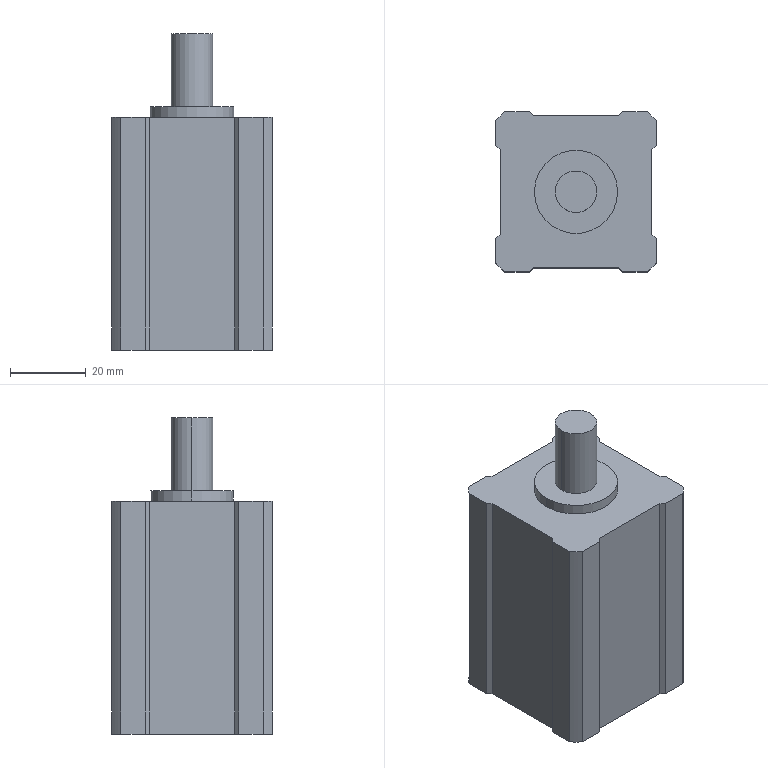Part | SolidWorks | features ICE 5, CirPattern 1, Extrusion 1, RefAxis 1, Scale 1 | 1 solid | 32 faces | box 42.35 x 42.35 x 83.6 mm | volume 106285 mm3 | plane 24 | cylinder 8 | commonest cylinder face diameters 56.65 x4 11 x2 22 x2
STEP:
#1=CARTESIAN_POINT('',(5.5,0.,109.667));
#2=VERTEX_POINT('',#1);
#3=CARTESIAN_POINT('',(-5.5,0.,109.667));
#4=VERTEX_POINT('',#3);
#5=CARTESIAN_POINT('',(0.,0.,109.667));
#6=DIRECTION('',(0.,0.,1.));
#7=DIRECTION('',(1.,0.,0.));
#8=AXIS2_PLACEMENT_3D('',#5,#6,#7);
#9=CIRCLE('',#8,5.5);
#10=EDGE_CURVE('',#2,#4,#9,.T.);
#11=ORIENTED_EDGE('',*,*,#10,.F.);
#12=CARTESIAN_POINT('',(5.5,0.,90.417));
#13=VERTEX_POINT('',#12);
#14=CARTESIAN_POINT('',(5.5,0.,109.667));
#15=DIRECTION('',(0.,0.,-1.));
#16=VECTOR('',#15,1000.);
#17=LINE('',#14,#16);
#18=EDGE_CURVE('',#2,#13,#17,.T.);
#19=ORIENTED_EDGE('',*,*,#18,.T.);
#20=CARTESIAN_POINT('',(-5.5,0.,90.417));
#21=VERTEX_POINT('',#20);
#22=CARTESIAN_POINT('',(0.,0.,90.417));
#23=DIRECTION('',(0.,0.,1.));
#24=DIRECTION('',(1.,0.,0.));
#25=AXIS2_PLACEMENT_3D('',#22,#23,#24);
#26=CIRCLE('',#25,5.5);
#27=EDGE_CURVE('',#13,#21,#26,.T.);
#28=ORIENTED_EDGE('',*,*,#27,.T.);
#29=CARTESIAN_POINT('',(-5.5,0.,109.667));
#30=DIRECTION('',(0.,0.,-1.));
#31=VECTOR('',#30,1000.);
#32=LINE('',#29,#31);
#33=EDGE_CURVE('',#4,#21,#32,.T.);
#34=ORIENTED_EDGE('',*,*,#33,.F.);
#35=EDGE_LOOP('',(#11,#19,#28,#34));
#36=FACE_OUTER_BOUND('',#35,.T.);
#37=CARTESIAN_POINT('',(0.,0.,109.667));
#38=DIRECTION('',(0.,0.,-1.));
#39=DIRECTION('',(-1.,0.,0.));
#40=AXIS2_PLACEMENT_3D('',#37,#38,#39);
#41=CYLINDRICAL_SURFACE('',#40,5.5);
#42=ADVANCED_FACE('',(#36),#41,.T.);
#43=CARTESIAN_POINT('',(11.,0.,90.417));
#44=VERTEX_POINT('',#43);
#45=CARTESIAN_POINT('',(-11.,0.,90.417));
#46=VERTEX_POINT('',#45);
#47=CARTESIAN_POINT('',(0.,0.,90.417));
#48=DIRECTION('',(0.,0.,1.));
#49=DIRECTION('',(1.,0.,0.));
#50=AXIS2_PLACEMENT_3D('',#47,#48,#49);
#51=CIRCLE('',#50,11.);
#52=EDGE_CURVE('',#44,#46,#51,.T.);
#53=ORIENTED_EDGE('',*,*,#52,.F.);
#54=CARTESIAN_POINT('',(11.,0.,87.667));
#55=VERTEX_POINT('',#54);
#56=CARTESIAN_POINT('',(11.,0.,90.417));
#57=DIRECTION('',(0.,0.,-1.));
#58=VECTOR('',#57,1000.);
#59=LINE('',#56,#58);
#60=EDGE_CURVE('',#44,#55,#59,.T.);
#61=ORIENTED_EDGE('',*,*,#60,.T.);
#62=CARTESIAN_POINT('',(-11.,0.,87.667));
#63=VERTEX_POINT('',#62);
#64=CARTESIAN_POINT('',(0.,0.,87.667));
#65=DIRECTION('',(0.,0.,1.));
#66=DIRECTION('',(1.,0.,0.));
#67=AXIS2_PLACEMENT_3D('',#64,#65,#66);
#68=CIRCLE('',#67,11.);
#69=EDGE_CURVE('',#55,#63,#68,.T.);
#70=ORIENTED_EDGE('',*,*,#69,.T.);
#71=CARTESIAN_POINT('',(-11.,0.,90.417));
#72=DIRECTION('',(0.,0.,-1.));
#73=VECTOR('',#72,1000.);
#74=LINE('',#71,#73);
#75=EDGE_CURVE('',#46,#63,#74,.T.);
#76=ORIENTED_EDGE('',*,*,#75,.F.);
#77=EDGE_LOOP('',(#53,#61,#70,#76));
#78=FACE_OUTER_BOUND('',#77,.T.);
#79=CARTESIAN_POINT('',(0.,0.,90.417));
#80=DIRECTION('',(0.,0.,-1.));
#81=DIRECTION('',(-1.,0.,0.));
#82=AXIS2_PLACEMENT_3D('',#79,#80,#81);
#83=CYLINDRICAL_SURFACE('',#82,11.);
#84=ADVANCED_FACE('',(#78),#83,.T.);
#85=CARTESIAN_POINT('',(21.175,12.375,87.667));
#86=VERTEX_POINT('',#85);
#87=CARTESIAN_POINT('',(20.075,11.275,87.667));
#88=VERTEX_POINT('',#87);
#89=CARTESIAN_POINT('',(21.175,12.375,87.667));
#90=DIRECTION('',(-0.7071,-0.7071,0.));
#91=VECTOR('',#90,1000.);
#92=LINE('',#89,#91);
#93=EDGE_CURVE('',#86,#88,#92,.T.);
#94=ORIENTED_EDGE('',*,*,#93,.F.);
#95=CARTESIAN_POINT('',(21.175,18.813,87.667));
#96=VERTEX_POINT('',#95);
#97=CARTESIAN_POINT('',(21.175,21.175,87.667));
#98=DIRECTION('',(0.,1.,0.));
#99=VECTOR('',#98,1000.);
#100=LINE('',#97,#99);
#101=EDGE_CURVE('',#86,#96,#100,.T.);
#102=ORIENTED_EDGE('',*,*,#101,.T.);
#103=CARTESIAN_POINT('',(18.813,21.175,87.667));
#104=VERTEX_POINT('',#103);
#105=CARTESIAN_POINT('',(0.,0.,87.667));
#106=DIRECTION('',(0.,0.,1.));
#107=DIRECTION('',(1.,0.,0.));
#108=AXIS2_PLACEMENT_3D('',#105,#106,#107);
#109=CIRCLE('',#108,28.325);
#110=EDGE_CURVE('',#96,#104,#109,.T.);
#111=ORIENTED_EDGE('',*,*,#110,.T.);
#112=CARTESIAN_POINT('',(12.375,21.175,87.667));
#113=VERTEX_POINT('',#112);
#114=CARTESIAN_POINT('',(-21.175,21.175,87.667));
#115=DIRECTION('',(-1.,0.,0.));
#116=VECTOR('',#115,1000.);
#117=LINE('',#114,#116);
#118=EDGE_CURVE('',#104,#113,#117,.T.);
#119=ORIENTED_EDGE('',*,*,#118,.T.);
#120=CARTESIAN_POINT('',(11.275,20.075,87.667));
#121=VERTEX_POINT('',#120);
#122=CARTESIAN_POINT('',(12.375,21.175,87.667));
#123=DIRECTION('',(0.7071,0.7071,0.));
#124=VECTOR('',#123,1000.);
#125=LINE('',#122,#124);
#126=EDGE_CURVE('',#121,#113,#125,.T.);
#127=ORIENTED_EDGE('',*,*,#126,.F.);
#128=CARTESIAN_POINT('',(-11.275,20.075,87.667));
#129=VERTEX_POINT('',#128);
#130=CARTESIAN_POINT('',(-11.275,20.075,87.667));
#131=DIRECTION('',(1.,0.,0.));
#132=VECTOR('',#131,1000.);
#133=LINE('',#130,#132);
#134=EDGE_CURVE('',#129,#121,#133,.T.);
#135=ORIENTED_EDGE('',*,*,#134,.F.);
#136=CARTESIAN_POINT('',(-12.375,21.175,87.667));
#137=VERTEX_POINT('',#136);
#138=CARTESIAN_POINT('',(-12.375,21.175,87.667));
#139=DIRECTION('',(0.7071,-0.7071,0.));
#140=VECTOR('',#139,1000.);
#141=LINE('',#138,#140);
#142=EDGE_CURVE('',#137,#129,#141,.T.);
#143=ORIENTED_EDGE('',*,*,#142,.F.);
#144=CARTESIAN_POINT('',(-18.813,21.175,87.667));
#145=VERTEX_POINT('',#144);
#146=CARTESIAN_POINT('',(-21.175,21.175,87.667));
#147=DIRECTION('',(-1.,0.,0.));
#148=VECTOR('',#147,1000.);
#149=LINE('',#146,#148);
#150=EDGE_CURVE('',#137,#145,#149,.T.);
#151=ORIENTED_EDGE('',*,*,#150,.T.);
#152=CARTESIAN_POINT('',(-21.175,18.813,87.667));
#153=VERTEX_POINT('',#152);
#154=CARTESIAN_POINT('',(0.,0.,87.667));
#155=DIRECTION('',(0.,0.,1.));
#156=DIRECTION('',(1.,0.,0.));
#157=AXIS2_PLACEMENT_3D('',#154,#155,#156);
#158=CIRCLE('',#157,28.325);
#159=EDGE_CURVE('',#145,#153,#158,.T.);
#160=ORIENTED_EDGE('',*,*,#159,.T.);
#161=CARTESIAN_POINT('',(-21.175,12.375,87.667));
#162=VERTEX_POINT('',#161);
#163=CARTESIAN_POINT('',(-21.175,21.175,87.667));
#164=DIRECTION('',(0.,-1.,0.));
#165=VECTOR('',#164,1000.);
#166=LINE('',#163,#165);
#167=EDGE_CURVE('',#153,#162,#166,.T.);
#168=ORIENTED_EDGE('',*,*,#167,.T.);
#169=CARTESIAN_POINT('',(-20.075,11.275,87.667));
#170=VERTEX_POINT('',#169);
#171=CARTESIAN_POINT('',(-21.175,12.375,87.667));
#172=DIRECTION('',(-0.7071,0.7071,0.));
#173=VECTOR('',#172,1000.);
#174=LINE('',#171,#173);
#175=EDGE_CURVE('',#170,#162,#174,.T.);
#176=ORIENTED_EDGE('',*,*,#175,.F.);
#177=CARTESIAN_POINT('',(-20.075,-11.275,87.667));
#178=VERTEX_POINT('',#177);
#179=CARTESIAN_POINT('',(-20.075,-11.275,87.667));
#180=DIRECTION('',(0.,1.,0.));
#181=VECTOR('',#180,1000.);
#182=LINE('',#179,#181);
#183=EDGE_CURVE('',#178,#170,#182,.T.);
#184=ORIENTED_EDGE('',*,*,#183,.F.);
#185=CARTESIAN_POINT('',(-21.175,-12.375,87.667));
#186=VERTEX_POINT('',#185);
#187=CARTESIAN_POINT('',(-21.175,-12.375,87.667));
#188=DIRECTION('',(0.7071,0.7071,0.));
#189=VECTOR('',#188,1000.);
#190=LINE('',#187,#189);
#191=EDGE_CURVE('',#186,#178,#190,.T.);
#192=ORIENTED_EDGE('',*,*,#191,.F.);
#193=CARTESIAN_POINT('',(-21.175,-18.813,87.667));
#194=VERTEX_POINT('',#193);
#195=CARTESIAN_POINT('',(-21.175,21.175,87.667));
#196=DIRECTION('',(0.,-1.,0.));
#197=VECTOR('',#196,1000.);
#198=LINE('',#195,#197);
#199=EDGE_CURVE('',#186,#194,#198,.T.);
#200=ORIENTED_EDGE('',*,*,#199,.T.);
#201=CARTESIAN_POINT('',(-18.813,-21.175,87.667));
#202=VERTEX_POINT('',#201);
#203=CARTESIAN_POINT('',(0.,0.,87.667));
#204=DIRECTION('',(0.,0.,1.));
#205=DIRECTION('',(1.,0.,0.));
#206=AXIS2_PLACEMENT_3D('',#203,#204,#205);
#207=CIRCLE('',#206,28.325);
#208=EDGE_CURVE('',#194,#202,#207,.T.);
#209=ORIENTED_EDGE('',*,*,#208,.T.);
#210=CARTESIAN_POINT('',(-12.375,-21.175,87.667));
#211=VERTEX_POINT('',#210);
#212=CARTESIAN_POINT('',(-21.175,-21.175,87.667));
#213=DIRECTION('',(1.,0.,0.));
#214=VECTOR('',#213,1000.);
#215=LINE('',#212,#214);
#216=EDGE_CURVE('',#202,#211,#215,.T.);
#217=ORIENTED_EDGE('',*,*,#216,.T.);
#218=CARTESIAN_POINT('',(-11.275,-20.075,87.667));
#219=VERTEX_POINT('',#218);
#220=CARTESIAN_POINT('',(-12.375,-21.175,87.667));
#221=DIRECTION('',(-0.7071,-0.7071,0.));
#222=VECTOR('',#221,1000.);
#223=LINE('',#220,#222);
#224=EDGE_CURVE('',#219,#211,#223,.T.);
#225=ORIENTED_EDGE('',*,*,#224,.F.);
#226=CARTESIAN_POINT('',(11.275,-20.075,87.667));
#227=VERTEX_POINT('',#226);
#228=CARTESIAN_POINT('',(11.275,-20.075,87.667));
#229=DIRECTION('',(-1.,0.,0.));
#230=VECTOR('',#229,1000.);
#231=LINE('',#228,#230);
#232=EDGE_CURVE('',#227,#219,#231,.T.);
#233=ORIENTED_EDGE('',*,*,#232,.F.);
#234=CARTESIAN_POINT('',(12.375,-21.175,87.667));
#235=VERTEX_POINT('',#234);
#236=CARTESIAN_POINT('',(12.375,-21.175,87.667));
#237=DIRECTION('',(-0.7071,0.7071,0.));
#238=VECTOR('',#237,1000.);
#239=LINE('',#236,#238);
#240=EDGE_CURVE('',#235,#227,#239,.T.);
#241=ORIENTED_EDGE('',*,*,#240,.F.);
#242=CARTESIAN_POINT('',(18.813,-21.175,87.667));
#243=VERTEX_POINT('',#242);
#244=CARTESIAN_POINT('',(-21.175,-21.175,87.667));
#245=DIRECTION('',(1.,0.,0.));
#246=VECTOR('',#245,1000.);
#247=LINE('',#244,#246);
#248=EDGE_CURVE('',#235,#243,#247,.T.);
#249=ORIENTED_EDGE('',*,*,#248,.T.);
#250=CARTESIAN_POINT('',(21.175,-18.813,87.667));
#251=VERTEX_POINT('',#250);
#252=CARTESIAN_POINT('',(0.,0.,87.667));
#253=DIRECTION('',(0.,0.,1.));
#254=DIRECTION('',(1.,0.,0.));
#255=AXIS2_PLACEMENT_3D('',#252,#253,#254);
#256=CIRCLE('',#255,28.325);
#257=EDGE_CURVE('',#243,#251,#256,.T.);
#258=ORIENTED_EDGE('',*,*,#257,.T.);
#259=CARTESIAN_POINT('',(21.175,-12.375,87.667));
#260=VERTEX_POINT('',#259);
#261=CARTESIAN_POINT('',(21.175,21.175,87.667));
#262=DIRECTION('',(0.,1.,0.));
#263=VECTOR('',#262,1000.);
#264=LINE('',#261,#263);
#265=EDGE_CURVE('',#251,#260,#264,.T.);
#266=ORIENTED_EDGE('',*,*,#265,.T.);
#267=CARTESIAN_POINT('',(20.075,-11.275,87.667));
#268=VERTEX_POINT('',#267);
#269=CARTESIAN_POINT('',(21.175,-12.375,87.667));
#270=DIRECTION('',(0.7071,-0.7071,0.));
#271=VECTOR('',#270,1000.);
#272=LINE('',#269,#271);
#273=EDGE_CURVE('',#268,#260,#272,.T.);
#274=ORIENTED_EDGE('',*,*,#273,.F.);
#275=CARTESIAN_POINT('',(20.075,11.275,87.667));
#276=DIRECTION('',(0.,-1.,0.));
#277=VECTOR('',#276,1000.);
#278=LINE('',#275,#277);
#279=EDGE_CURVE('',#88,#268,#278,.T.);
#280=ORIENTED_EDGE('',*,*,#279,.F.);
#281=EDGE_LOOP('',(#94,#102,#111,#119,#127,#135,#143,#151,#160,#168,#176,#184,#192,#200,#209,#217,#225,#233,#241,#249,#258,#266,#274,#280));
#282=FACE_OUTER_BOUND('',#281,.T.);
#283=CARTESIAN_POINT('',(0.,0.,87.667));
#284=DIRECTION('',(0.,0.,1.));
#285=DIRECTION('',(1.,0.,0.));
#286=AXIS2_PLACEMENT_3D('',#283,#284,#285);
#287=CIRCLE('',#286,11.);
#288=EDGE_CURVE('',#63,#55,#287,.T.);
#289=ORIENTED_EDGE('',*,*,#288,.F.);
#290=ORIENTED_EDGE('',*,*,#69,.F.);
#291=EDGE_LOOP('',(#289,#290));
#292=FACE_BOUND('',#291,.T.);
#293=CARTESIAN_POINT('',(21.175,-21.175,87.667));
#294=DIRECTION('',(0.,0.,1.));
#295=DIRECTION('',(1.,0.,0.));
#296=AXIS2_PLACEMENT_3D('',#293,#294,#295);
#297=PLANE('',#296);
#298=ADVANCED_FACE('',(#282,#292),#297,.T.);
#299=ORIENTED_EDGE('',*,*,#101,.F.);
#300=CARTESIAN_POINT('',(21.175,12.375,26.067));
#301=VERTEX_POINT('',#300);
#302=CARTESIAN_POINT('',(21.175,12.375,26.067));
#303=DIRECTION('',(0.,0.,1.));
#304=VECTOR('',#303,1000.);
#305=LINE('',#302,#304);
#306=EDGE_CURVE('',#301,#86,#305,.T.);
#307=ORIENTED_EDGE('',*,*,#306,.F.);
#308=CARTESIAN_POINT('',(21.175,18.813,26.067));
#309=VERTEX_POINT('',#308);
#310=CARTESIAN_POINT('',(21.175,21.175,26.067));
#311=DIRECTION('',(0.,1.,0.));
#312=VECTOR('',#311,1000.);
#313=LINE('',#310,#312);
#314=EDGE_CURVE('',#301,#309,#313,.T.);
#315=ORIENTED_EDGE('',*,*,#314,.T.);
#316=CARTESIAN_POINT('',(21.175,18.813,26.067));
#317=DIRECTION('',(0.,0.,-1.));
#318=VECTOR('',#317,1000.);
#319=LINE('',#316,#318);
#320=EDGE_CURVE('',#96,#309,#319,.T.);
#321=ORIENTED_EDGE('',*,*,#320,.F.);
#322=EDGE_LOOP('',(#299,#307,#315,#321));
#323=FACE_OUTER_BOUND('',#322,.T.);
#324=CARTESIAN_POINT('',(21.175,21.175,87.667));
#325=DIRECTION('',(-1.,0.,0.));
#326=DIRECTION('',(0.,-1.,0.));
#327=AXIS2_PLACEMENT_3D('',#324,#325,#326);
#328=PLANE('',#327);
#329=ADVANCED_FACE('',(#323),#328,.F.);
#330=ORIENTED_EDGE('',*,*,#248,.F.);
#331=CARTESIAN_POINT('',(12.375,-21.175,26.067));
#332=VERTEX_POINT('',#331);
#333=CARTESIAN_POINT('',(12.375,-21.175,26.067));
#334=DIRECTION('',(0.,0.,1.));
#335=VECTOR('',#334,1000.);
#336=LINE('',#333,#335);
#337=EDGE_CURVE('',#332,#235,#336,.T.);
#338=ORIENTED_EDGE('',*,*,#337,.F.);
#339=CARTESIAN_POINT('',(18.813,-21.175,26.067));
#340=VERTEX_POINT('',#339);
#341=CARTESIAN_POINT('',(-21.175,-21.175,26.067));
#342=DIRECTION('',(1.,0.,0.));
#343=VECTOR('',#342,1000.);
#344=LINE('',#341,#343);
#345=EDGE_CURVE('',#332,#340,#344,.T.);
#346=ORIENTED_EDGE('',*,*,#345,.T.);
#347=CARTESIAN_POINT('',(18.813,-21.175,26.067));
#348=DIRECTION('',(0.,0.,-1.));
#349=VECTOR('',#348,1000.);
#350=LINE('',#347,#349);
#351=EDGE_CURVE('',#243,#340,#350,.T.);
#352=ORIENTED_EDGE('',*,*,#351,.F.);
#353=EDGE_LOOP('',(#330,#338,#346,#352));
#354=FACE_OUTER_BOUND('',#353,.T.);
#355=CARTESIAN_POINT('',(-21.175,-21.175,87.667));
#356=DIRECTION('',(0.,1.,0.));
#357=DIRECTION('',(0.,0.,1.));
#358=AXIS2_PLACEMENT_3D('',#355,#356,#357);
#359=PLANE('',#358);
#360=ADVANCED_FACE('',(#354),#359,.F.);
#361=ORIENTED_EDGE('',*,*,#199,.F.);
#362=CARTESIAN_POINT('',(-21.175,-12.375,26.067));
#363=VERTEX_POINT('',#362);
#364=CARTESIAN_POINT('',(-21.175,-12.375,26.067));
#365=DIRECTION('',(0.,0.,1.));
#366=VECTOR('',#365,1000.);
#367=LINE('',#364,#366);
#368=EDGE_CURVE('',#363,#186,#367,.T.);
#369=ORIENTED_EDGE('',*,*,#368,.F.);
#370=CARTESIAN_POINT('',(-21.175,-18.813,26.067));
#371=VERTEX_POINT('',#370);
#372=CARTESIAN_POINT('',(-21.175,21.175,26.067));
#373=DIRECTION('',(0.,-1.,0.));
#374=VECTOR('',#373,1000.);
#375=LINE('',#372,#374);
#376=EDGE_CURVE('',#363,#371,#375,.T.);
#377=ORIENTED_EDGE('',*,*,#376,.T.);
#378=CARTESIAN_POINT('',(-21.175,-18.813,26.067));
#379=DIRECTION('',(0.,0.,-1.));
#380=VECTOR('',#379,1000.);
#381=LINE('',#378,#380);
#382=EDGE_CURVE('',#194,#371,#381,.T.);
#383=ORIENTED_EDGE('',*,*,#382,.F.);
#384=EDGE_LOOP('',(#361,#369,#377,#383));
#385=FACE_OUTER_BOUND('',#384,.T.);
#386=CARTESIAN_POINT('',(-21.175,21.175,87.667));
#387=DIRECTION('',(1.,0.,0.));
#388=DIRECTION('',(0.,0.,-1.));
#389=AXIS2_PLACEMENT_3D('',#386,#387,#388);
#390=PLANE('',#389);
#391=ADVANCED_FACE('',(#385),#390,.F.);
#392=ORIENTED_EDGE('',*,*,#150,.F.);
#393=CARTESIAN_POINT('',(-12.375,21.175,26.067));
#394=VERTEX_POINT('',#393);
#395=CARTESIAN_POINT('',(-12.375,21.175,26.067));
#396=DIRECTION('',(0.,0.,1.));
#397=VECTOR('',#396,1000.);
#398=LINE('',#395,#397);
#399=EDGE_CURVE('',#394,#137,#398,.T.);
#400=ORIENTED_EDGE('',*,*,#399,.F.);
#401=CARTESIAN_POINT('',(-18.813,21.175,26.067));
#402=VERTEX_POINT('',#401);
#403=CARTESIAN_POINT('',(-21.175,21.175,26.067));
#404=DIRECTION('',(-1.,0.,0.));
#405=VECTOR('',#404,1000.);
#406=LINE('',#403,#405);
#407=EDGE_CURVE('',#394,#402,#406,.T.);
#408=ORIENTED_EDGE('',*,*,#407,.T.);
#409=CARTESIAN_POINT('',(-18.813,21.175,26.067));
#410=DIRECTION('',(0.,0.,-1.));
#411=VECTOR('',#410,1000.);
#412=LINE('',#409,#411);
#413=EDGE_CURVE('',#145,#402,#412,.T.);
#414=ORIENTED_EDGE('',*,*,#413,.F.);
#415=EDGE_LOOP('',(#392,#400,#408,#414));
#416=FACE_OUTER_BOUND('',#415,.T.);
#417=CARTESIAN_POINT('',(-21.175,21.175,87.667));
#418=DIRECTION('',(0.,-1.,0.));
#419=DIRECTION('',(0.,0.,-1.));
#420=AXIS2_PLACEMENT_3D('',#417,#418,#419);
#421=PLANE('',#420);
#422=ADVANCED_FACE('',(#416),#421,.F.);
#423=CARTESIAN_POINT('',(21.175,-18.813,26.067));
#424=VERTEX_POINT('',#423);
#425=CARTESIAN_POINT('',(21.175,-12.375,26.067));
#426=VERTEX_POINT('',#425);
#427=CARTESIAN_POINT('',(21.175,21.175,26.067));
#428=DIRECTION('',(0.,1.,0.));
#429=VECTOR('',#428,1000.);
#430=LINE('',#427,#429);
#431=EDGE_CURVE('',#424,#426,#430,.T.);
#432=ORIENTED_EDGE('',*,*,#431,.T.);
#433=CARTESIAN_POINT('',(21.175,-12.375,26.067));
#434=DIRECTION('',(0.,0.,1.));
#435=VECTOR('',#434,1000.);
#436=LINE('',#433,#435);
#437=EDGE_CURVE('',#426,#260,#436,.T.);
#438=ORIENTED_EDGE('',*,*,#437,.T.);
#439=ORIENTED_EDGE('',*,*,#265,.F.);
#440=CARTESIAN_POINT('',(21.175,-18.813,26.067));
#441=DIRECTION('',(0.,0.,1.));
#442=VECTOR('',#441,1000.);
#443=LINE('',#440,#442);
#444=EDGE_CURVE('',#424,#251,#443,.T.);
#445=ORIENTED_EDGE('',*,*,#444,.F.);
#446=EDGE_LOOP('',(#432,#438,#439,#445));
#447=FACE_OUTER_BOUND('',#446,.T.);
#448=CARTESIAN_POINT('',(21.175,21.175,87.667));
#449=DIRECTION('',(-1.,0.,0.));
#450=DIRECTION('',(0.,-1.,0.));
#451=AXIS2_PLACEMENT_3D('',#448,#449,#450);
#452=PLANE('',#451);
#453=ADVANCED_FACE('',(#447),#452,.F.);
#454=CARTESIAN_POINT('',(18.813,21.175,26.067));
#455=VERTEX_POINT('',#454);
#456=CARTESIAN_POINT('',(12.375,21.175,26.067));
#457=VERTEX_POINT('',#456);
#458=CARTESIAN_POINT('',(-21.175,21.175,26.067));
#459=DIRECTION('',(-1.,0.,0.));
#460=VECTOR('',#459,1000.);
#461=LINE('',#458,#460);
#462=EDGE_CURVE('',#455,#457,#461,.T.);
#463=ORIENTED_EDGE('',*,*,#462,.T.);
#464=CARTESIAN_POINT('',(12.375,21.175,26.067));
#465=DIRECTION('',(0.,0.,1.));
#466=VECTOR('',#465,1000.);
#467=LINE('',#464,#466);
#468=EDGE_CURVE('',#457,#113,#467,.T.);
#469=ORIENTED_EDGE('',*,*,#468,.T.);
#470=ORIENTED_EDGE('',*,*,#118,.F.);
#471=CARTESIAN_POINT('',(18.813,21.175,26.067));
#472=DIRECTION('',(0.,0.,1.));
#473=VECTOR('',#472,1000.);
#474=LINE('',#471,#473);
#475=EDGE_CURVE('',#455,#104,#474,.T.);
#476=ORIENTED_EDGE('',*,*,#475,.F.);
#477=EDGE_LOOP('',(#463,#469,#470,#476));
#478=FACE_OUTER_BOUND('',#477,.T.);
#479=CARTESIAN_POINT('',(-21.175,21.175,87.667));
#480=DIRECTION('',(0.,-1.,0.));
#481=DIRECTION('',(0.,0.,-1.));
#482=AXIS2_PLACEMENT_3D('',#479,#480,#481);
#483=PLANE('',#482);
#484=ADVANCED_FACE('',(#478),#483,.F.);
#485=CARTESIAN_POINT('',(-21.175,18.813,26.067));
#486=VERTEX_POINT('',#485);
#487=CARTESIAN_POINT('',(-21.175,12.375,26.067));
#488=VERTEX_POINT('',#487);
#489=CARTESIAN_POINT('',(-21.175,21.175,26.067));
#490=DIRECTION('',(0.,-1.,0.));
#491=VECTOR('',#490,1000.);
#492=LINE('',#489,#491);
#493=EDGE_CURVE('',#486,#488,#492,.T.);
#494=ORIENTED_EDGE('',*,*,#493,.T.);
#495=CARTESIAN_POINT('',(-21.175,12.375,26.067));
#496=DIRECTION('',(0.,0.,1.));
#497=VECTOR('',#496,1000.);
#498=LINE('',#495,#497);
#499=EDGE_CURVE('',#488,#162,#498,.T.);
#500=ORIENTED_EDGE('',*,*,#499,.T.);
#501=ORIENTED_EDGE('',*,*,#167,.F.);
#502=CARTESIAN_POINT('',(-21.175,18.813,26.067));
#503=DIRECTION('',(0.,0.,1.));
#504=VECTOR('',#503,1000.);
#505=LINE('',#502,#504);
#506=EDGE_CURVE('',#486,#153,#505,.T.);
#507=ORIENTED_EDGE('',*,*,#506,.F.);
#508=EDGE_LOOP('',(#494,#500,#501,#507));
#509=FACE_OUTER_BOUND('',#508,.T.);
#510=CARTESIAN_POINT('',(-21.175,21.175,87.667));
#511=DIRECTION('',(1.,0.,0.));
#512=DIRECTION('',(0.,0.,-1.));
#513=AXIS2_PLACEMENT_3D('',#510,#511,#512);
#514=PLANE('',#513);
#515=ADVANCED_FACE('',(#509),#514,.F.);
#516=CARTESIAN_POINT('',(-18.813,-21.175,26.067));
#517=VERTEX_POINT('',#516);
#518=CARTESIAN_POINT('',(-12.375,-21.175,26.067));
#519=VERTEX_POINT('',#518);
#520=CARTESIAN_POINT('',(-21.175,-21.175,26.067));
#521=DIRECTION('',(1.,0.,0.));
#522=VECTOR('',#521,1000.);
#523=LINE('',#520,#522);
#524=EDGE_CURVE('',#517,#519,#523,.T.);
#525=ORIENTED_EDGE('',*,*,#524,.T.);
#526=CARTESIAN_POINT('',(-12.375,-21.175,26.067));
#527=DIRECTION('',(0.,0.,1.));
#528=VECTOR('',#527,1000.);
#529=LINE('',#526,#528);
#530=EDGE_CURVE('',#519,#211,#529,.T.);
#531=ORIENTED_EDGE('',*,*,#530,.T.);
#532=ORIENTED_EDGE('',*,*,#216,.F.);
#533=CARTESIAN_POINT('',(-18.813,-21.175,26.067));
#534=DIRECTION('',(0.,0.,1.));
#535=VECTOR('',#534,1000.);
#536=LINE('',#533,#535);
#537=EDGE_CURVE('',#517,#202,#536,.T.);
#538=ORIENTED_EDGE('',*,*,#537,.F.);
#539=EDGE_LOOP('',(#525,#531,#532,#538));
#540=FACE_OUTER_BOUND('',#539,.T.);
#541=CARTESIAN_POINT('',(-21.175,-21.175,87.667));
#542=DIRECTION('',(0.,1.,0.));
#543=DIRECTION('',(0.,0.,1.));
#544=AXIS2_PLACEMENT_3D('',#541,#542,#543);
#545=PLANE('',#544);
#546=ADVANCED_FACE('',(#540),#545,.F.);
#547=ORIENTED_EDGE('',*,*,#314,.F.);
#548=CARTESIAN_POINT('',(20.075,11.275,26.067));
#549=VERTEX_POINT('',#548);
#550=CARTESIAN_POINT('',(21.175,12.375,26.067));
#551=DIRECTION('',(-0.7071,-0.7071,0.));
#552=VECTOR('',#551,1000.);
#553=LINE('',#550,#552);
#554=EDGE_CURVE('',#301,#549,#553,.T.);
#555=ORIENTED_EDGE('',*,*,#554,.T.);
#556=CARTESIAN_POINT('',(20.075,-11.275,26.067));
#557=VERTEX_POINT('',#556);
#558=CARTESIAN_POINT('',(20.075,11.275,26.067));
#559=DIRECTION('',(0.,-1.,0.));
#560=VECTOR('',#559,1000.);
#561=LINE('',#558,#560);
#562=EDGE_CURVE('',#549,#557,#561,.T.);
#563=ORIENTED_EDGE('',*,*,#562,.T.);
#564=CARTESIAN_POINT('',(21.175,-12.375,26.067));
#565=DIRECTION('',(0.7071,-0.7071,0.));
#566=VECTOR('',#565,1000.);
#567=LINE('',#564,#566);
#568=EDGE_CURVE('',#557,#426,#567,.T.);
#569=ORIENTED_EDGE('',*,*,#568,.T.);
#570=ORIENTED_EDGE('',*,*,#431,.F.);
#571=CARTESIAN_POINT('',(0.,0.,26.067));
#572=DIRECTION('',(0.,0.,1.));
#573=DIRECTION('',(1.,0.,0.));
#574=AXIS2_PLACEMENT_3D('',#571,#572,#573);
#575=CIRCLE('',#574,28.325);
#576=EDGE_CURVE('',#340,#424,#575,.T.);
#577=ORIENTED_EDGE('',*,*,#576,.F.);
#578=ORIENTED_EDGE('',*,*,#345,.F.);
#579=CARTESIAN_POINT('',(11.275,-20.075,26.067));
#580=VERTEX_POINT('',#579);
#581=CARTESIAN_POINT('',(12.375,-21.175,26.067));
#582=DIRECTION('',(-0.7071,0.7071,0.));
#583=VECTOR('',#582,1000.);
#584=LINE('',#581,#583);
#585=EDGE_CURVE('',#332,#580,#584,.T.);
#586=ORIENTED_EDGE('',*,*,#585,.T.);
#587=CARTESIAN_POINT('',(-11.275,-20.075,26.067));
#588=VERTEX_POINT('',#587);
#589=CARTESIAN_POINT('',(11.275,-20.075,26.067));
#590=DIRECTION('',(-1.,0.,0.));
#591=VECTOR('',#590,1000.);
#592=LINE('',#589,#591);
#593=EDGE_CURVE('',#580,#588,#592,.T.);
#594=ORIENTED_EDGE('',*,*,#593,.T.);
#595=CARTESIAN_POINT('',(-12.375,-21.175,26.067));
#596=DIRECTION('',(-0.7071,-0.7071,0.));
#597=VECTOR('',#596,1000.);
#598=LINE('',#595,#597);
#599=EDGE_CURVE('',#588,#519,#598,.T.);
#600=ORIENTED_EDGE('',*,*,#599,.T.);
#601=ORIENTED_EDGE('',*,*,#524,.F.);
#602=CARTESIAN_POINT('',(0.,0.,26.067));
#603=DIRECTION('',(0.,0.,1.));
#604=DIRECTION('',(1.,0.,0.));
#605=AXIS2_PLACEMENT_3D('',#602,#603,#604);
#606=CIRCLE('',#605,28.325);
#607=EDGE_CURVE('',#371,#517,#606,.T.);
#608=ORIENTED_EDGE('',*,*,#607,.F.);
#609=ORIENTED_EDGE('',*,*,#376,.F.);
#610=CARTESIAN_POINT('',(-20.075,-11.275,26.067));
#611=VERTEX_POINT('',#610);
#612=CARTESIAN_POINT('',(-21.175,-12.375,26.067));
#613=DIRECTION('',(0.7071,0.7071,0.));
#614=VECTOR('',#613,1000.);
#615=LINE('',#612,#614);
#616=EDGE_CURVE('',#363,#611,#615,.T.);
#617=ORIENTED_EDGE('',*,*,#616,.T.);
#618=CARTESIAN_POINT('',(-20.075,11.275,26.067));
#619=VERTEX_POINT('',#618);
#620=CARTESIAN_POINT('',(-20.075,-11.275,26.067));
#621=DIRECTION('',(0.,1.,0.));
#622=VECTOR('',#621,1000.);
#623=LINE('',#620,#622);
#624=EDGE_CURVE('',#611,#619,#623,.T.);
#625=ORIENTED_EDGE('',*,*,#624,.T.);
#626=CARTESIAN_POINT('',(-21.175,12.375,26.067));
#627=DIRECTION('',(-0.7071,0.7071,0.));
#628=VECTOR('',#627,1000.);
#629=LINE('',#626,#628);
#630=EDGE_CURVE('',#619,#488,#629,.T.);
#631=ORIENTED_EDGE('',*,*,#630,.T.);
#632=ORIENTED_EDGE('',*,*,#493,.F.);
#633=CARTESIAN_POINT('',(0.,0.,26.067));
#634=DIRECTION('',(0.,0.,1.));
#635=DIRECTION('',(1.,0.,0.));
#636=AXIS2_PLACEMENT_3D('',#633,#634,#635);
#637=CIRCLE('',#636,28.325);
#638=EDGE_CURVE('',#402,#486,#637,.T.);
#639=ORIENTED_EDGE('',*,*,#638,.F.);
#640=ORIENTED_EDGE('',*,*,#407,.F.);
#641=CARTESIAN_POINT('',(-11.275,20.075,26.067));
#642=VERTEX_POINT('',#641);
#643=CARTESIAN_POINT('',(-12.375,21.175,26.067));
#644=DIRECTION('',(0.7071,-0.7071,0.));
#645=VECTOR('',#644,1000.);
#646=LINE('',#643,#645);
#647=EDGE_CURVE('',#394,#642,#646,.T.);
#648=ORIENTED_EDGE('',*,*,#647,.T.);
#649=CARTESIAN_POINT('',(11.275,20.075,26.067));
#650=VERTEX_POINT('',#649);
#651=CARTESIAN_POINT('',(-11.275,20.075,26.067));
#652=DIRECTION('',(1.,0.,0.));
#653=VECTOR('',#652,1000.);
#654=LINE('',#651,#653);
#655=EDGE_CURVE('',#642,#650,#654,.T.);
#656=ORIENTED_EDGE('',*,*,#655,.T.);
#657=CARTESIAN_POINT('',(12.375,21.175,26.067));
#658=DIRECTION('',(0.7071,0.7071,0.));
#659=VECTOR('',#658,1000.);
#660=LINE('',#657,#659);
#661=EDGE_CURVE('',#650,#457,#660,.T.);
#662=ORIENTED_EDGE('',*,*,#661,.T.);
#663=ORIENTED_EDGE('',*,*,#462,.F.);
#664=CARTESIAN_POINT('',(0.,0.,26.067));
#665=DIRECTION('',(0.,0.,1.));
#666=DIRECTION('',(1.,0.,0.));
#667=AXIS2_PLACEMENT_3D('',#664,#665,#666);
#668=CIRCLE('',#667,28.325);
#669=EDGE_CURVE('',#309,#455,#668,.T.);
#670=ORIENTED_EDGE('',*,*,#669,.F.);
#671=EDGE_LOOP('',(#547,#555,#563,#569,#570,#577,#578,#586,#594,#600,#601,#608,#609,#617,#625,#631,#632,#639,#640,#648,#656,#662,#663,#670));
#672=FACE_OUTER_BOUND('',#671,.T.);
#673=CARTESIAN_POINT('',(21.175,-21.175,26.067));
#674=DIRECTION('',(0.,0.,1.));
#675=DIRECTION('',(1.,0.,0.));
#676=AXIS2_PLACEMENT_3D('',#673,#674,#675);
#677=PLANE('',#676);
#678=ADVANCED_FACE('',(#672),#677,.F.);
#679=ORIENTED_EDGE('',*,*,#444,.T.);
#680=ORIENTED_EDGE('',*,*,#257,.F.);
#681=ORIENTED_EDGE('',*,*,#351,.T.);
#682=ORIENTED_EDGE('',*,*,#576,.T.);
#683=EDGE_LOOP('',(#679,#680,#681,#682));
#684=FACE_OUTER_BOUND('',#683,.T.);
#685=CARTESIAN_POINT('',(0.,0.,26.067));
#686=DIRECTION('',(0.,0.,1.));
#687=DIRECTION('',(1.,0.,0.));
#688=AXIS2_PLACEMENT_3D('',#685,#686,#687);
#689=CYLINDRICAL_SURFACE('',#688,28.325);
#690=ADVANCED_FACE('',(#684),#689,.T.);
#691=ORIENTED_EDGE('',*,*,#382,.T.);
#692=ORIENTED_EDGE('',*,*,#607,.T.);
#693=ORIENTED_EDGE('',*,*,#537,.T.);
#694=ORIENTED_EDGE('',*,*,#208,.F.);
#695=EDGE_LOOP('',(#691,#692,#693,#694));
#696=FACE_OUTER_BOUND('',#695,.T.);
#697=CARTESIAN_POINT('',(0.,0.,26.067));
#698=DIRECTION('',(0.,0.,1.));
#699=DIRECTION('',(1.,0.,0.));
#700=AXIS2_PLACEMENT_3D('',#697,#698,#699);
#701=CYLINDRICAL_SURFACE('',#700,28.325);
#702=ADVANCED_FACE('',(#696),#701,.T.);
#703=ORIENTED_EDGE('',*,*,#413,.T.);
#704=ORIENTED_EDGE('',*,*,#638,.T.);
#705=ORIENTED_EDGE('',*,*,#506,.T.);
#706=ORIENTED_EDGE('',*,*,#159,.F.);
#707=EDGE_LOOP('',(#703,#704,#705,#706));
#708=FACE_OUTER_BOUND('',#707,.T.);
#709=CARTESIAN_POINT('',(0.,0.,26.067));
#710=DIRECTION('',(0.,0.,1.));
#711=DIRECTION('',(1.,0.,0.));
#712=AXIS2_PLACEMENT_3D('',#709,#710,#711);
#713=CYLINDRICAL_SURFACE('',#712,28.325);
#714=ADVANCED_FACE('',(#708),#713,.T.);
#715=ORIENTED_EDGE('',*,*,#320,.T.);
#716=ORIENTED_EDGE('',*,*,#669,.T.);
#717=ORIENTED_EDGE('',*,*,#475,.T.);
#718=ORIENTED_EDGE('',*,*,#110,.F.);
#719=EDGE_LOOP('',(#715,#716,#717,#718));
#720=FACE_OUTER_BOUND('',#719,.T.);
#721=CARTESIAN_POINT('',(0.,0.,26.067));
#722=DIRECTION('',(0.,0.,1.));
#723=DIRECTION('',(1.,0.,0.));
#724=AXIS2_PLACEMENT_3D('',#721,#722,#723);
#725=CYLINDRICAL_SURFACE('',#724,28.325);
#726=ADVANCED_FACE('',(#720),#725,.T.);
#727=ORIENTED_EDGE('',*,*,#142,.T.);
#728=CARTESIAN_POINT('',(-11.275,20.075,26.067));
#729=DIRECTION('',(0.,0.,1.));
#730=VECTOR('',#729,1000.);
#731=LINE('',#728,#730);
#732=EDGE_CURVE('',#642,#129,#731,.T.);
#733=ORIENTED_EDGE('',*,*,#732,.F.);
#734=ORIENTED_EDGE('',*,*,#647,.F.);
#735=ORIENTED_EDGE('',*,*,#399,.T.);
#736=EDGE_LOOP('',(#727,#733,#734,#735));
#737=FACE_OUTER_BOUND('',#736,.T.);
#738=CARTESIAN_POINT('',(-12.375,21.175,26.067));
#739=DIRECTION('',(-0.7071,-0.7071,0.));
#740=DIRECTION('',(0.7071,-0.7071,0.));
#741=AXIS2_PLACEMENT_3D('',#738,#739,#740);
#742=PLANE('',#741);
#743=ADVANCED_FACE('',(#737),#742,.F.);
#744=ORIENTED_EDGE('',*,*,#126,.T.);
#745=ORIENTED_EDGE('',*,*,#468,.F.);
#746=ORIENTED_EDGE('',*,*,#661,.F.);
#747=CARTESIAN_POINT('',(11.275,20.075,26.067));
#748=DIRECTION('',(0.,0.,1.));
#749=VECTOR('',#748,1000.);
#750=LINE('',#747,#749);
#751=EDGE_CURVE('',#650,#121,#750,.T.);
#752=ORIENTED_EDGE('',*,*,#751,.T.);
#753=EDGE_LOOP('',(#744,#745,#746,#752));
#754=FACE_OUTER_BOUND('',#753,.T.);
#755=CARTESIAN_POINT('',(12.375,21.175,26.067));
#756=DIRECTION('',(0.7071,-0.7071,0.));
#757=DIRECTION('',(0.7071,0.7071,0.));
#758=AXIS2_PLACEMENT_3D('',#755,#756,#757);
#759=PLANE('',#758);
#760=ADVANCED_FACE('',(#754),#759,.F.);
#761=ORIENTED_EDGE('',*,*,#134,.T.);
#762=ORIENTED_EDGE('',*,*,#751,.F.);
#763=ORIENTED_EDGE('',*,*,#655,.F.);
#764=ORIENTED_EDGE('',*,*,#732,.T.);
#765=EDGE_LOOP('',(#761,#762,#763,#764));
#766=FACE_OUTER_BOUND('',#765,.T.);
#767=CARTESIAN_POINT('',(-11.275,20.075,26.067));
#768=DIRECTION('',(0.,-1.,0.));
#769=DIRECTION('',(1.,0.,0.));
#770=AXIS2_PLACEMENT_3D('',#767,#768,#769);
#771=PLANE('',#770);
#772=ADVANCED_FACE('',(#766),#771,.F.);
#773=ORIENTED_EDGE('',*,*,#191,.T.);
#774=CARTESIAN_POINT('',(-20.075,-11.275,26.067));
#775=DIRECTION('',(0.,0.,1.));
#776=VECTOR('',#775,1000.);
#777=LINE('',#774,#776);
#778=EDGE_CURVE('',#611,#178,#777,.T.);
#779=ORIENTED_EDGE('',*,*,#778,.F.);
#780=ORIENTED_EDGE('',*,*,#616,.F.);
#781=ORIENTED_EDGE('',*,*,#368,.T.);
#782=EDGE_LOOP('',(#773,#779,#780,#781));
#783=FACE_OUTER_BOUND('',#782,.T.);
#784=CARTESIAN_POINT('',(-21.175,-12.375,26.067));
#785=DIRECTION('',(0.7071,-0.7071,0.));
#786=DIRECTION('',(0.7071,0.7071,0.));
#787=AXIS2_PLACEMENT_3D('',#784,#785,#786);
#788=PLANE('',#787);
#789=ADVANCED_FACE('',(#783),#788,.F.);
#790=ORIENTED_EDGE('',*,*,#175,.T.);
#791=ORIENTED_EDGE('',*,*,#499,.F.);
#792=ORIENTED_EDGE('',*,*,#630,.F.);
#793=CARTESIAN_POINT('',(-20.075,11.275,26.067));
#794=DIRECTION('',(0.,0.,1.));
#795=VECTOR('',#794,1000.);
#796=LINE('',#793,#795);
#797=EDGE_CURVE('',#619,#170,#796,.T.);
#798=ORIENTED_EDGE('',*,*,#797,.T.);
#799=EDGE_LOOP('',(#790,#791,#792,#798));
#800=FACE_OUTER_BOUND('',#799,.T.);
#801=CARTESIAN_POINT('',(-21.175,12.375,26.067));
#802=DIRECTION('',(0.7071,0.7071,0.));
#803=DIRECTION('',(-0.7071,0.7071,0.));
#804=AXIS2_PLACEMENT_3D('',#801,#802,#803);
#805=PLANE('',#804);
#806=ADVANCED_FACE('',(#800),#805,.F.);
#807=ORIENTED_EDGE('',*,*,#183,.T.);
#808=ORIENTED_EDGE('',*,*,#797,.F.);
#809=ORIENTED_EDGE('',*,*,#624,.F.);
#810=ORIENTED_EDGE('',*,*,#778,.T.);
#811=EDGE_LOOP('',(#807,#808,#809,#810));
#812=FACE_OUTER_BOUND('',#811,.T.);
#813=CARTESIAN_POINT('',(-20.075,-11.275,26.067));
#814=DIRECTION('',(1.,0.,0.));
#815=DIRECTION('',(0.,1.,0.));
#816=AXIS2_PLACEMENT_3D('',#813,#814,#815);
#817=PLANE('',#816);
#818=ADVANCED_FACE('',(#812),#817,.F.);
#819=ORIENTED_EDGE('',*,*,#240,.T.);
#820=CARTESIAN_POINT('',(11.275,-20.075,26.067));
#821=DIRECTION('',(0.,0.,1.));
#822=VECTOR('',#821,1000.);
#823=LINE('',#820,#822);
#824=EDGE_CURVE('',#580,#227,#823,.T.);
#825=ORIENTED_EDGE('',*,*,#824,.F.);
#826=ORIENTED_EDGE('',*,*,#585,.F.);
#827=ORIENTED_EDGE('',*,*,#337,.T.);
#828=EDGE_LOOP('',(#819,#825,#826,#827));
#829=FACE_OUTER_BOUND('',#828,.T.);
#830=CARTESIAN_POINT('',(12.375,-21.175,26.067));
#831=DIRECTION('',(0.7071,0.7071,0.));
#832=DIRECTION('',(-0.7071,0.7071,0.));
#833=AXIS2_PLACEMENT_3D('',#830,#831,#832);
#834=PLANE('',#833);
#835=ADVANCED_FACE('',(#829),#834,.F.);
#836=ORIENTED_EDGE('',*,*,#224,.T.);
#837=ORIENTED_EDGE('',*,*,#530,.F.);
#838=ORIENTED_EDGE('',*,*,#599,.F.);
#839=CARTESIAN_POINT('',(-11.275,-20.075,26.067));
#840=DIRECTION('',(0.,0.,1.));
#841=VECTOR('',#840,1000.);
#842=LINE('',#839,#841);
#843=EDGE_CURVE('',#588,#219,#842,.T.);
#844=ORIENTED_EDGE('',*,*,#843,.T.);
#845=EDGE_LOOP('',(#836,#837,#838,#844));
#846=FACE_OUTER_BOUND('',#845,.T.);
#847=CARTESIAN_POINT('',(-12.375,-21.175,26.067));
#848=DIRECTION('',(-0.7071,0.7071,0.));
#849=DIRECTION('',(-0.7071,-0.7071,0.));
#850=AXIS2_PLACEMENT_3D('',#847,#848,#849);
#851=PLANE('',#850);
#852=ADVANCED_FACE('',(#846),#851,.F.);
#853=ORIENTED_EDGE('',*,*,#232,.T.);
#854=ORIENTED_EDGE('',*,*,#843,.F.);
#855=ORIENTED_EDGE('',*,*,#593,.F.);
#856=ORIENTED_EDGE('',*,*,#824,.T.);
#857=EDGE_LOOP('',(#853,#854,#855,#856));
#858=FACE_OUTER_BOUND('',#857,.T.);
#859=CARTESIAN_POINT('',(11.275,-20.075,26.067));
#860=DIRECTION('',(0.,1.,0.));
#861=DIRECTION('',(-1.,0.,0.));
#862=AXIS2_PLACEMENT_3D('',#859,#860,#861);
#863=PLANE('',#862);
#864=ADVANCED_FACE('',(#858),#863,.F.);
#865=ORIENTED_EDGE('',*,*,#93,.T.);
#866=CARTESIAN_POINT('',(20.075,11.275,26.067));
#867=DIRECTION('',(0.,0.,1.));
#868=VECTOR('',#867,1000.);
#869=LINE('',#866,#868);
#870=EDGE_CURVE('',#549,#88,#869,.T.);
#871=ORIENTED_EDGE('',*,*,#870,.F.);
#872=ORIENTED_EDGE('',*,*,#554,.F.);
#873=ORIENTED_EDGE('',*,*,#306,.T.);
#874=EDGE_LOOP('',(#865,#871,#872,#873));
#875=FACE_OUTER_BOUND('',#874,.T.);
#876=CARTESIAN_POINT('',(21.175,12.375,26.067));
#877=DIRECTION('',(-0.7071,0.7071,0.));
#878=DIRECTION('',(-0.7071,-0.7071,0.));
#879=AXIS2_PLACEMENT_3D('',#876,#877,#878);
#880=PLANE('',#879);
#881=ADVANCED_FACE('',(#875),#880,.F.);
#882=ORIENTED_EDGE('',*,*,#273,.T.);
#883=ORIENTED_EDGE('',*,*,#437,.F.);
#884=ORIENTED_EDGE('',*,*,#568,.F.);
#885=CARTESIAN_POINT('',(20.075,-11.275,26.067));
#886=DIRECTION('',(0.,0.,1.));
#887=VECTOR('',#886,1000.);
#888=LINE('',#885,#887);
#889=EDGE_CURVE('',#557,#268,#888,.T.);
#890=ORIENTED_EDGE('',*,*,#889,.T.);
#891=EDGE_LOOP('',(#882,#883,#884,#890));
#892=FACE_OUTER_BOUND('',#891,.T.);
#893=CARTESIAN_POINT('',(21.175,-12.375,26.067));
#894=DIRECTION('',(-0.7071,-0.7071,0.));
#895=DIRECTION('',(0.7071,-0.7071,0.));
#896=AXIS2_PLACEMENT_3D('',#893,#894,#895);
#897=PLANE('',#896);
#898=ADVANCED_FACE('',(#892),#897,.F.);
#899=ORIENTED_EDGE('',*,*,#279,.T.);
#900=ORIENTED_EDGE('',*,*,#889,.F.);
#901=ORIENTED_EDGE('',*,*,#562,.F.);
#902=ORIENTED_EDGE('',*,*,#870,.T.);
#903=EDGE_LOOP('',(#899,#900,#901,#902));
#904=FACE_OUTER_BOUND('',#903,.T.);
#905=CARTESIAN_POINT('',(20.075,11.275,26.067));
#906=DIRECTION('',(-1.,0.,0.));
#907=DIRECTION('',(0.,-1.,0.));
#908=AXIS2_PLACEMENT_3D('',#905,#906,#907);
#909=PLANE('',#908);
#910=ADVANCED_FACE('',(#904),#909,.F.);
#911=CARTESIAN_POINT('',(0.,0.,90.417));
#912=DIRECTION('',(0.,0.,1.));
#913=DIRECTION('',(1.,0.,0.));
#914=AXIS2_PLACEMENT_3D('',#911,#912,#913);
#915=CIRCLE('',#914,11.);
#916=EDGE_CURVE('',#46,#44,#915,.T.);
#917=ORIENTED_EDGE('',*,*,#916,.T.);
#918=ORIENTED_EDGE('',*,*,#52,.T.);
#919=EDGE_LOOP('',(#917,#918));
#920=FACE_OUTER_BOUND('',#919,.T.);
#921=CARTESIAN_POINT('',(0.,0.,90.417));
#922=DIRECTION('',(0.,0.,1.));
#923=DIRECTION('',(1.,0.,0.));
#924=AXIS2_PLACEMENT_3D('',#921,#922,#923);
#925=CIRCLE('',#924,5.5);
#926=EDGE_CURVE('',#21,#13,#925,.T.);
#927=ORIENTED_EDGE('',*,*,#926,.F.);
#928=ORIENTED_EDGE('',*,*,#27,.F.);
#929=EDGE_LOOP('',(#927,#928));
#930=FACE_BOUND('',#929,.T.);
#931=CARTESIAN_POINT('',(0.,0.,90.417));
#932=DIRECTION('',(0.,0.,1.));
#933=DIRECTION('',(1.,0.,0.));
#934=AXIS2_PLACEMENT_3D('',#931,#932,#933);
#935=PLANE('',#934);
#936=ADVANCED_FACE('',(#920,#930),#935,.T.);
#937=ORIENTED_EDGE('',*,*,#60,.F.);
#938=ORIENTED_EDGE('',*,*,#916,.F.);
#939=ORIENTED_EDGE('',*,*,#75,.T.);
#940=ORIENTED_EDGE('',*,*,#288,.T.);
#941=EDGE_LOOP('',(#937,#938,#939,#940));
#942=FACE_OUTER_BOUND('',#941,.T.);
#943=CARTESIAN_POINT('',(0.,0.,90.417));
#944=DIRECTION('',(0.,0.,-1.));
#945=DIRECTION('',(-1.,0.,0.));
#946=AXIS2_PLACEMENT_3D('',#943,#944,#945);
#947=CYLINDRICAL_SURFACE('',#946,11.);
#948=ADVANCED_FACE('',(#942),#947,.T.);
#949=ORIENTED_EDGE('',*,*,#18,.F.);
#950=CARTESIAN_POINT('',(0.,0.,109.667));
#951=DIRECTION('',(0.,0.,1.));
#952=DIRECTION('',(1.,0.,0.));
#953=AXIS2_PLACEMENT_3D('',#950,#951,#952);
#954=CIRCLE('',#953,5.5);
#955=EDGE_CURVE('',#4,#2,#954,.T.);
#956=ORIENTED_EDGE('',*,*,#955,.F.);
#957=ORIENTED_EDGE('',*,*,#33,.T.);
#958=ORIENTED_EDGE('',*,*,#926,.T.);
#959=EDGE_LOOP('',(#949,#956,#957,#958));
#960=FACE_OUTER_BOUND('',#959,.T.);
#961=CARTESIAN_POINT('',(0.,0.,109.667));
#962=DIRECTION('',(0.,0.,-1.));
#963=DIRECTION('',(-1.,0.,0.));
#964=AXIS2_PLACEMENT_3D('',#961,#962,#963);
#965=CYLINDRICAL_SURFACE('',#964,5.5);
#966=ADVANCED_FACE('',(#960),#965,.T.);
#967=ORIENTED_EDGE('',*,*,#955,.T.);
#968=ORIENTED_EDGE('',*,*,#10,.T.);
#969=EDGE_LOOP('',(#967,#968));
#970=FACE_OUTER_BOUND('',#969,.T.);
#971=CARTESIAN_POINT('',(0.,0.,109.667));
#972=DIRECTION('',(0.,0.,1.));
#973=DIRECTION('',(1.,0.,0.));
#974=AXIS2_PLACEMENT_3D('',#971,#972,#973);
#975=PLANE('',#974);
#976=ADVANCED_FACE('',(#970),#975,.T.);
#977=CLOSED_SHELL('',(#42,#84,#298,#329,#360,#391,#422,#453,#484,#515,#546,#678,#690,#702,#714,#726,#743,#760,#772,#789,#806,#818,#835,#852,#864,#881,#898,#910,#936,#948,#966,#976));
#978=MANIFOLD_SOLID_BREP('',#977);
#979=CARTESIAN_POINT('',(0.,0.,0.));
#980=DIRECTION('',(0.,0.,1.));
#981=DIRECTION('',(1.,0.,0.));
#982=AXIS2_PLACEMENT_3D('',#979,#980,#981);
#983=(LENGTH_UNIT()NAMED_UNIT(*)SI_UNIT(.MILLI.,.METRE.));
#984=UNCERTAINTY_MEASURE_WITH_UNIT(LENGTH_MEASURE(0.00001),#983,'','');
#985=(NAMED_UNIT(*)PLANE_ANGLE_UNIT()SI_UNIT($,.RADIAN.));
#986=(NAMED_UNIT(*)SI_UNIT($,.STERADIAN.)SOLID_ANGLE_UNIT());
#987=(GEOMETRIC_REPRESENTATION_CONTEXT(3)GLOBAL_UNCERTAINTY_ASSIGNED_CONTEXT((#984))GLOBAL_UNIT_ASSIGNED_CONTEXT((#983,#985,#986))REPRESENTATION_CONTEXT('',''));
#988=ADVANCED_BREP_SHAPE_REPRESENTATION('',(#978,#982),#987);